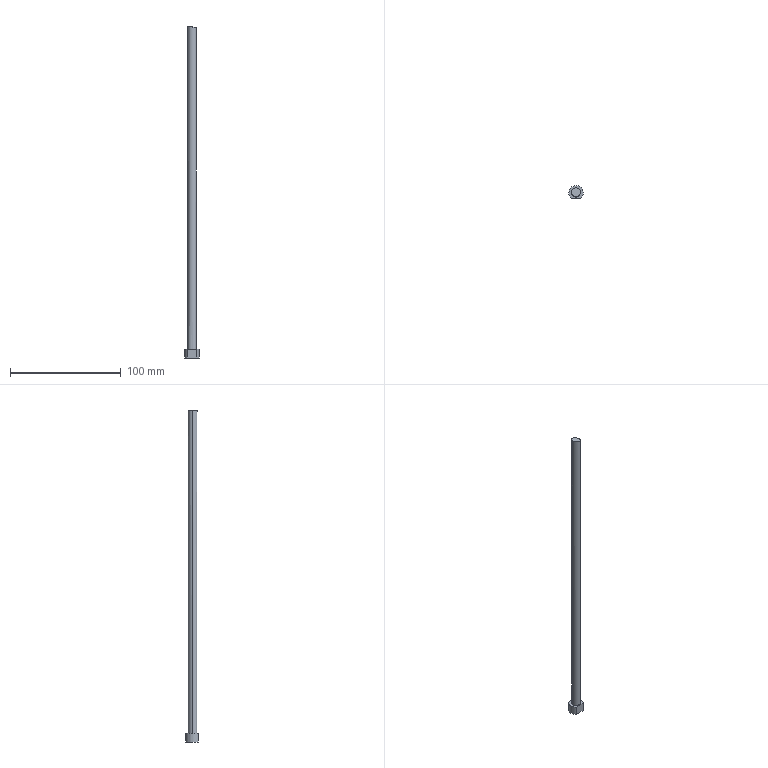Part | Creo | 1 solid | 7 faces | box 13 x 11.5 x 300.057 mm | volume 15631 mm3 | plane 4 | cylinder 3 | commonest cylinder face diameters 8 x2 13 x1
STEP:
#1=CARTESIAN_POINT('',(56.,-18.,2.356));
#2=VERTEX_POINT('',#1);
#3=CARTESIAN_POINT('',(48.,-18.,4.057));
#4=VERTEX_POINT('',#3);
#5=CARTESIAN_POINT('',(56.,-18.,2.356));
#6=CARTESIAN_POINT('',(56.,-18.384,2.356));
#7=CARTESIAN_POINT('',(55.895,-19.121,2.379));
#8=CARTESIAN_POINT('',(55.421,-20.178,2.48));
#9=CARTESIAN_POINT('',(54.668,-21.054,2.64));
#10=CARTESIAN_POINT('',(53.693,-21.686,2.847));
#11=CARTESIAN_POINT('',(52.564,-22.017,3.087));
#12=CARTESIAN_POINT('',(51.394,-22.011,3.335));
#13=CARTESIAN_POINT('',(50.274,-21.67,3.574));
#14=CARTESIAN_POINT('',(49.314,-21.036,3.778));
#15=CARTESIAN_POINT('',(48.573,-20.167,3.935));
#16=CARTESIAN_POINT('',(48.106,-19.119,4.034));
#17=CARTESIAN_POINT('',(48.,-18.384,4.057));
#18=CARTESIAN_POINT('',(48.,-18.,4.057));
#19=B_SPLINE_CURVE_WITH_KNOTS('',3,(#5,#6,#7,#8,#9,#10,#11,#12,#13,#14,#15,#16,#17,#18),.UNSPECIFIED.,.F.,.F.,(4,1,1,1,1,1,1,1,1,1,1,4),(0.,0.09091,0.1818,0.2727,0.3636,0.4545,0.5455,0.6364,0.7273,0.8182,0.9091,1.),.UNSPECIFIED.);
#20=EDGE_CURVE('',#2,#4,#19,.T.);
#21=ORIENTED_EDGE('',*,*,#20,.T.);
#22=CARTESIAN_POINT('',(48.,-18.,4.057));
#23=CARTESIAN_POINT('',(48.,-17.616,4.057));
#24=CARTESIAN_POINT('',(48.105,-16.879,4.035));
#25=CARTESIAN_POINT('',(48.579,-15.822,3.934));
#26=CARTESIAN_POINT('',(49.332,-14.946,3.774));
#27=CARTESIAN_POINT('',(50.307,-14.314,3.567));
#28=CARTESIAN_POINT('',(51.436,-13.983,3.327));
#29=CARTESIAN_POINT('',(52.606,-13.989,3.078));
#30=CARTESIAN_POINT('',(53.726,-14.33,2.84));
#31=CARTESIAN_POINT('',(54.686,-14.964,2.636));
#32=CARTESIAN_POINT('',(55.427,-15.833,2.478));
#33=CARTESIAN_POINT('',(55.894,-16.88,2.379));
#34=CARTESIAN_POINT('',(56.,-17.616,2.356));
#35=CARTESIAN_POINT('',(56.,-18.,2.356));
#36=B_SPLINE_CURVE_WITH_KNOTS('',3,(#22,#23,#24,#25,#26,#27,#28,#29,#30,#31,#32,#33,#34,#35),.UNSPECIFIED.,.F.,.F.,(4,1,1,1,1,1,1,1,1,1,1,4),(0.,0.09091,0.1818,0.2727,0.3636,0.4545,0.5455,0.6364,0.7273,0.8182,0.9091,1.),.UNSPECIFIED.);
#37=EDGE_CURVE('',#4,#2,#36,.T.);
#38=ORIENTED_EDGE('',*,*,#37,.T.);
#39=EDGE_LOOP('',(#21,#38));
#40=FACE_OUTER_BOUND('',#39,.F.);
#41=CARTESIAN_POINT('',(58.154,-132.981,1.899));
#42=DIRECTION('',(-0.2079,0.000000129,-0.9781));
#43=DIRECTION('',(0.000000618,1.,0.));
#44=AXIS2_PLACEMENT_3D('',#41,#42,#43);
#45=PLANE('',#44);
#46=ADVANCED_FACE('',(#40),#45,.F.);
#47=CARTESIAN_POINT('',(56.,-18.,-288.));
#48=VERTEX_POINT('',#47);
#49=CARTESIAN_POINT('',(48.,-18.,-288.));
#50=VERTEX_POINT('',#49);
#51=CARTESIAN_POINT('',(52.,-18.,-288.));
#52=DIRECTION('',(0.,0.,-1.));
#53=DIRECTION('',(1.,0.,0.));
#54=AXIS2_PLACEMENT_3D('',#51,#52,#53);
#55=CIRCLE('',#54,4.);
#56=EDGE_CURVE('',#48,#50,#55,.T.);
#57=ORIENTED_EDGE('',*,*,#56,.T.);
#58=CARTESIAN_POINT('',(48.,-18.,-288.));
#59=DIRECTION('',(0.,0.000000003,1.));
#60=VECTOR('',#59,292.057);
#61=LINE('',#58,#60);
#62=EDGE_CURVE('',#50,#4,#61,.T.);
#63=ORIENTED_EDGE('',*,*,#62,.T.);
#64=ORIENTED_EDGE('',*,*,#20,.F.);
#65=CARTESIAN_POINT('',(56.,-18.,-288.));
#66=DIRECTION('',(0.,-0.000000003,1.));
#67=VECTOR('',#66,290.356);
#68=LINE('',#65,#67);
#69=EDGE_CURVE('',#48,#2,#68,.T.);
#70=ORIENTED_EDGE('',*,*,#69,.F.);
#71=EDGE_LOOP('',(#57,#63,#64,#70));
#72=FACE_OUTER_BOUND('',#71,.F.);
#73=CARTESIAN_POINT('',(52.,-18.,-385.948));
#74=DIRECTION('',(0.,0.,1.));
#75=DIRECTION('',(1.,0.,0.));
#76=AXIS2_PLACEMENT_3D('',#73,#74,#75);
#77=CYLINDRICAL_SURFACE('',#76,4.);
#78=ADVANCED_FACE('',(#72),#77,.T.);
#79=CARTESIAN_POINT('',(47.847,-23.,-288.));
#80=VERTEX_POINT('',#79);
#81=CARTESIAN_POINT('',(56.153,-23.,-288.));
#82=VERTEX_POINT('',#81);
#83=CARTESIAN_POINT('',(47.847,-23.,-288.));
#84=DIRECTION('',(1.,0.,0.));
#85=VECTOR('',#84,8.307);
#86=LINE('',#83,#85);
#87=EDGE_CURVE('',#80,#82,#86,.T.);
#88=ORIENTED_EDGE('',*,*,#87,.F.);
#89=CARTESIAN_POINT('',(45.5,-18.,-288.));
#90=VERTEX_POINT('',#89);
#91=CARTESIAN_POINT('',(52.,-18.,-288.));
#92=DIRECTION('',(0.,0.,1.));
#93=DIRECTION('',(-1.,0.,0.));
#94=AXIS2_PLACEMENT_3D('',#91,#92,#93);
#95=CIRCLE('',#94,6.5);
#96=EDGE_CURVE('',#90,#80,#95,.T.);
#97=ORIENTED_EDGE('',*,*,#96,.F.);
#98=CARTESIAN_POINT('',(52.,-18.,-288.));
#99=DIRECTION('',(0.,0.,1.));
#100=DIRECTION('',(0.639,-0.7692,0.));
#101=AXIS2_PLACEMENT_3D('',#98,#99,#100);
#102=CIRCLE('',#101,6.5);
#103=EDGE_CURVE('',#82,#90,#102,.T.);
#104=ORIENTED_EDGE('',*,*,#103,.F.);
#105=EDGE_LOOP('',(#88,#97,#104));
#106=FACE_OUTER_BOUND('',#105,.F.);
#107=ORIENTED_EDGE('',*,*,#56,.F.);
#108=CARTESIAN_POINT('',(52.,-18.,-288.));
#109=DIRECTION('',(0.,0.,-1.));
#110=DIRECTION('',(-1.,0.,0.));
#111=AXIS2_PLACEMENT_3D('',#108,#109,#110);
#112=CIRCLE('',#111,4.);
#113=EDGE_CURVE('',#50,#48,#112,.T.);
#114=ORIENTED_EDGE('',*,*,#113,.F.);
#115=EDGE_LOOP('',(#107,#114));
#116=FACE_BOUND('',#115,.F.);
#117=CARTESIAN_POINT('',(52.,-18.,-288.));
#118=DIRECTION('',(0.,0.,1.));
#119=DIRECTION('',(-1.,0.,0.));
#120=AXIS2_PLACEMENT_3D('',#117,#118,#119);
#121=PLANE('',#120);
#122=ADVANCED_FACE('',(#106,#116),#121,.T.);
#123=CARTESIAN_POINT('',(47.847,-23.,-296.));
#124=VERTEX_POINT('',#123);
#125=CARTESIAN_POINT('',(47.847,-23.,-296.));
#126=DIRECTION('',(0.,0.,1.));
#127=VECTOR('',#126,8.);
#128=LINE('',#125,#127);
#129=EDGE_CURVE('',#124,#80,#128,.T.);
#130=ORIENTED_EDGE('',*,*,#129,.T.);
#131=ORIENTED_EDGE('',*,*,#87,.T.);
#132=CARTESIAN_POINT('',(56.153,-23.,-296.));
#133=VERTEX_POINT('',#132);
#134=CARTESIAN_POINT('',(56.153,-23.,-288.));
#135=DIRECTION('',(0.,0.,-1.));
#136=VECTOR('',#135,8.);
#137=LINE('',#134,#136);
#138=EDGE_CURVE('',#82,#133,#137,.T.);
#139=ORIENTED_EDGE('',*,*,#138,.T.);
#140=CARTESIAN_POINT('',(47.847,-23.,-296.));
#141=DIRECTION('',(1.,0.,0.));
#142=VECTOR('',#141,8.307);
#143=LINE('',#140,#142);
#144=EDGE_CURVE('',#124,#133,#143,.T.);
#145=ORIENTED_EDGE('',*,*,#144,.F.);
#146=EDGE_LOOP('',(#130,#131,#139,#145));
#147=FACE_OUTER_BOUND('',#146,.F.);
#148=CARTESIAN_POINT('',(52.,-23.,-296.));
#149=DIRECTION('',(0.,1.,0.));
#150=DIRECTION('',(0.,0.,-1.));
#151=AXIS2_PLACEMENT_3D('',#148,#149,#150);
#152=PLANE('',#151);
#153=ADVANCED_FACE('',(#147),#152,.F.);
#154=ORIENTED_EDGE('',*,*,#129,.F.);
#155=CARTESIAN_POINT('',(45.5,-18.,-296.));
#156=VERTEX_POINT('',#155);
#157=CARTESIAN_POINT('',(52.,-18.,-296.));
#158=DIRECTION('',(0.,0.,-1.));
#159=DIRECTION('',(-0.639,-0.7692,0.));
#160=AXIS2_PLACEMENT_3D('',#157,#158,#159);
#161=CIRCLE('',#160,6.5);
#162=EDGE_CURVE('',#124,#156,#161,.T.);
#163=ORIENTED_EDGE('',*,*,#162,.T.);
#164=CARTESIAN_POINT('',(52.,-18.,-296.));
#165=DIRECTION('',(0.,0.,-1.));
#166=DIRECTION('',(-1.,0.,0.));
#167=AXIS2_PLACEMENT_3D('',#164,#165,#166);
#168=CIRCLE('',#167,6.5);
#169=EDGE_CURVE('',#156,#133,#168,.T.);
#170=ORIENTED_EDGE('',*,*,#169,.T.);
#171=ORIENTED_EDGE('',*,*,#138,.F.);
#172=ORIENTED_EDGE('',*,*,#103,.T.);
#173=ORIENTED_EDGE('',*,*,#96,.T.);
#174=EDGE_LOOP('',(#154,#163,#170,#171,#172,#173));
#175=FACE_OUTER_BOUND('',#174,.F.);
#176=CARTESIAN_POINT('',(52.,-18.,-296.));
#177=DIRECTION('',(0.,0.,1.));
#178=DIRECTION('',(-1.,0.,0.));
#179=AXIS2_PLACEMENT_3D('',#176,#177,#178);
#180=CYLINDRICAL_SURFACE('',#179,6.5);
#181=ADVANCED_FACE('',(#175),#180,.T.);
#182=ORIENTED_EDGE('',*,*,#162,.F.);
#183=ORIENTED_EDGE('',*,*,#144,.T.);
#184=ORIENTED_EDGE('',*,*,#169,.F.);
#185=EDGE_LOOP('',(#182,#183,#184));
#186=FACE_OUTER_BOUND('',#185,.F.);
#187=CARTESIAN_POINT('',(10.,-36.005,-296.));
#188=DIRECTION('',(0.,0.,1.));
#189=DIRECTION('',(0.,1.,0.));
#190=AXIS2_PLACEMENT_3D('',#187,#188,#189);
#191=PLANE('',#190);
#192=ADVANCED_FACE('',(#186),#191,.F.);
#193=ORIENTED_EDGE('',*,*,#113,.T.);
#194=ORIENTED_EDGE('',*,*,#69,.T.);
#195=ORIENTED_EDGE('',*,*,#37,.F.);
#196=ORIENTED_EDGE('',*,*,#62,.F.);
#197=EDGE_LOOP('',(#193,#194,#195,#196));
#198=FACE_OUTER_BOUND('',#197,.F.);
#199=CARTESIAN_POINT('',(52.,-18.,-385.948));
#200=DIRECTION('',(0.,0.,1.));
#201=DIRECTION('',(1.,0.,0.));
#202=AXIS2_PLACEMENT_3D('',#199,#200,#201);
#203=CYLINDRICAL_SURFACE('',#202,4.);
#204=ADVANCED_FACE('',(#198),#203,.T.);
#205=CLOSED_SHELL('',(#46,#78,#122,#153,#181,#192,#204));
#206=MANIFOLD_SOLID_BREP('',#205);
#207=(LENGTH_UNIT()NAMED_UNIT(*)SI_UNIT(.MILLI.,.METRE.));
#208=UNCERTAINTY_MEASURE_WITH_UNIT(LENGTH_MEASURE(0.03005),#207,'','');
#209=(NAMED_UNIT(*)PLANE_ANGLE_UNIT()SI_UNIT($,.RADIAN.));
#210=PLANE_ANGLE_MEASURE_WITH_UNIT(PLANE_ANGLE_MEASURE(0.01745),#209);
#211=(CONVERSION_BASED_UNIT('DEGREE',#210)NAMED_UNIT(*)PLANE_ANGLE_UNIT());
#212=(NAMED_UNIT(*)SI_UNIT($,.STERADIAN.)SOLID_ANGLE_UNIT());
#213=(GEOMETRIC_REPRESENTATION_CONTEXT(3)GLOBAL_UNCERTAINTY_ASSIGNED_CONTEXT((#208))GLOBAL_UNIT_ASSIGNED_CONTEXT((#207,#211,#212))REPRESENTATION_CONTEXT('',''));
#214=ADVANCED_BREP_SHAPE_REPRESENTATION('',(#206),#213);